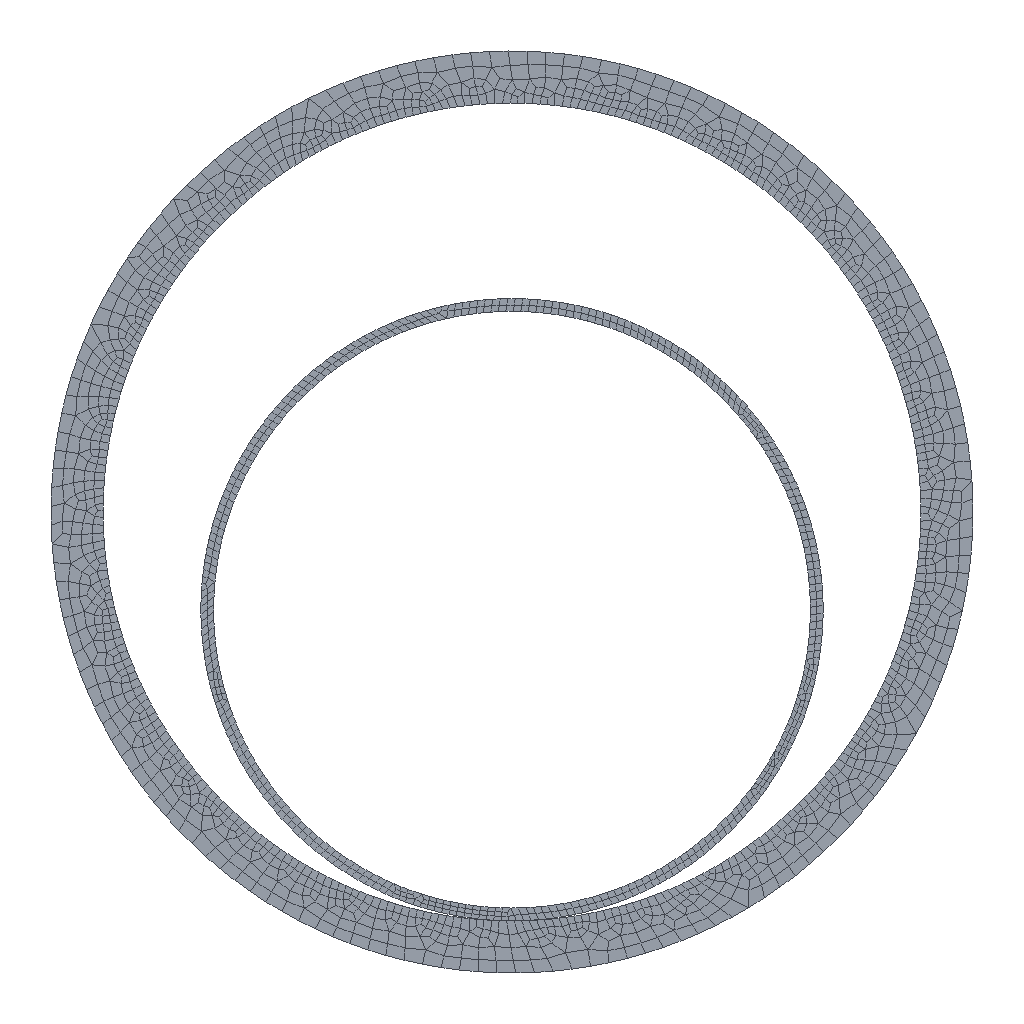Simulation study | abaqus
Set-up summary:
category,name,step,type,value,unit,region
solver,abaqus
solver,version,,,Abaqus/Standard 3DEXPERIENCE R2017x
units,not stated in the deck,,not stated
analysis,deck,,static,static
load_step,Step-1,Step-1,static,nlgeom=True
load_step,Step-2,Step-2,static,nlgeom=True
contact,interactions,,,general=0 pairs=1 ties=0
load_step,requested,,,2
mesh,nodes,,,2378
mesh,elements,,,1875
element_type,CPE4,,plane,1875
load,load commands in deck,,count,4
bc,support commands in deck,,count,4
material,MATERIAL-2,,in results
material,STEEL,,in results
check,setup vs results,,match,"per instance, exact: element labels, types and connectivity; labels of the nodes the elements use; coordinates of those nodes at SINGLE_PRECISION in 2 of 2 instance(s)"
Results summary:
result,step,,partial,increments=23 time=1/1.0
result,step,,completed,increments=97 time=36000.0/36000.0
result,analysis,,,static
result,last_loadstep,,,2
result,analysis steps,,count,2
result,primary field,,,U
result,reaction total,,FX,165.505,model units
result,reaction total,,FY,10021.592,model units
result,reaction total,,FZ,0.0,model units